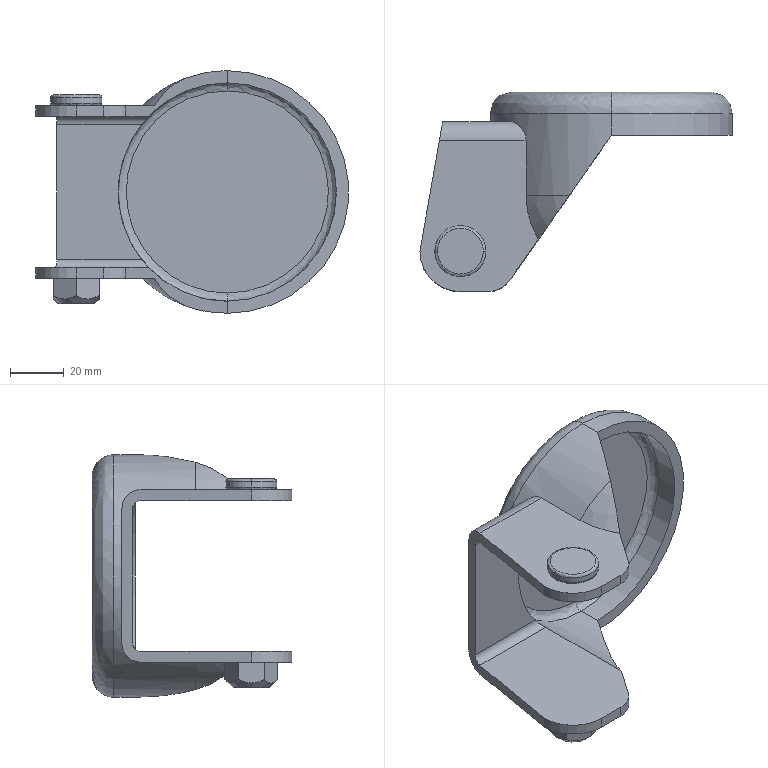Part | STEP file | CDAN75-Mb | 1 solid | 48 faces | box 116 x 74 x 90 mm | volume 70869 mm3 | plane 22 | cylinder 14 | spline 10 | cone 2 | commonest cylinder face diameters 6 x2 14 x2 19 x2 20 x2 30 x2 81 x2